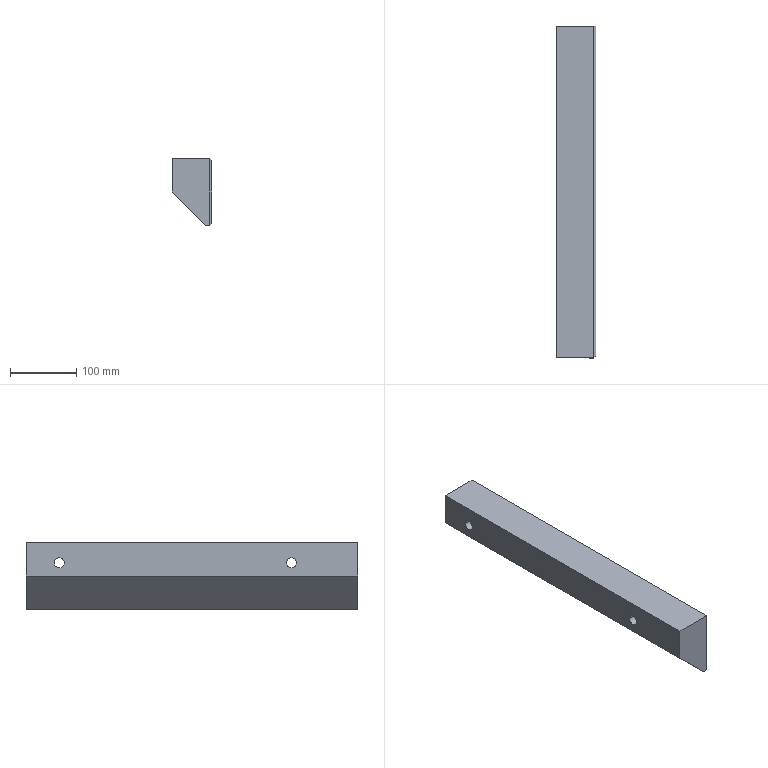Part | SolidWorks | features BaseBody 1 | 1 solid | 18 faces | box 60 x 500 x 100 mm | volume 2348382 mm3 | plane 10 | cone 4 | cylinder 4 | commonest cylinder face diameters 15 x4
STEP:
#1=CARTESIAN_POINT('',(125.077,156.249,507.107));
#2=VERTEX_POINT('',#1);
#3=CARTESIAN_POINT('',(122.077,153.249,510.107));
#4=VERTEX_POINT('',#3);
#5=CARTESIAN_POINT('',(257.41,288.582,374.773));
#6=DIRECTION('',(-0.5774,-0.5774,0.5774));
#7=VECTOR('',#6,1000.);
#8=LINE('',#5,#7);
#9=EDGE_CURVE('',#2,#4,#8,.T.);
#10=ORIENTED_EDGE('',*,*,#9,.T.);
#11=CARTESIAN_POINT('',(122.077,153.249,410.107));
#12=VERTEX_POINT('',#11);
#13=CARTESIAN_POINT('',(122.077,153.249,510.107));
#14=DIRECTION('',(0.,0.,1.));
#15=VECTOR('',#14,1000.);
#16=LINE('',#13,#15);
#17=EDGE_CURVE('',#12,#4,#16,.T.);
#18=ORIENTED_EDGE('',*,*,#17,.F.);
#19=CARTESIAN_POINT('',(125.077,156.249,413.107));
#20=VERTEX_POINT('',#19);
#21=CARTESIAN_POINT('',(124.077,155.249,412.107));
#22=DIRECTION('',(-0.5774,-0.5774,-0.5774));
#23=VECTOR('',#22,1000.);
#24=LINE('',#21,#23);
#25=EDGE_CURVE('',#20,#12,#24,.T.);
#26=ORIENTED_EDGE('',*,*,#25,.F.);
#27=CARTESIAN_POINT('',(125.077,156.249,410.107));
#28=DIRECTION('',(0.,0.,-1.));
#29=VECTOR('',#28,1000.);
#30=LINE('',#27,#29);
#31=EDGE_CURVE('',#2,#20,#30,.T.);
#32=ORIENTED_EDGE('',*,*,#31,.F.);
#33=EDGE_LOOP('',(#10,#18,#26,#32));
#34=FACE_OUTER_BOUND('',#33,.T.);
#35=CARTESIAN_POINT('',(125.077,156.249,410.107));
#36=DIRECTION('',(0.7071,-0.7071,0.));
#37=DIRECTION('',(0.,0.,-1.));
#38=AXIS2_PLACEMENT_3D('',#35,#36,#37);
#39=PLANE('',#38);
#40=ADVANCED_FACE('',(#34),#39,.T.);
#41=CARTESIAN_POINT('',(122.077,260.749,480.107));
#42=VERTEX_POINT('',#41);
#43=CARTESIAN_POINT('',(122.077,245.749,480.107));
#44=VERTEX_POINT('',#43);
#45=CARTESIAN_POINT('',(122.077,253.249,480.107));
#46=DIRECTION('',(1.,0.,0.));
#47=DIRECTION('',(0.,1.,0.));
#48=AXIS2_PLACEMENT_3D('',#45,#46,#47);
#49=CIRCLE('',#48,7.5);
#50=EDGE_CURVE('',#42,#44,#49,.T.);
#51=ORIENTED_EDGE('',*,*,#50,.F.);
#52=CARTESIAN_POINT('',(125.077,263.749,480.107));
#53=VERTEX_POINT('',#52);
#54=CARTESIAN_POINT('',(122.077,260.749,480.107));
#55=DIRECTION('',(0.7071,0.7071,0.));
#56=VECTOR('',#55,1000.);
#57=LINE('',#54,#56);
#58=EDGE_CURVE('',#42,#53,#57,.T.);
#59=ORIENTED_EDGE('',*,*,#58,.T.);
#60=CARTESIAN_POINT('',(125.077,242.749,480.107));
#61=VERTEX_POINT('',#60);
#62=CARTESIAN_POINT('',(125.077,253.249,480.107));
#63=DIRECTION('',(-1.,0.,0.));
#64=DIRECTION('',(0.,1.,0.));
#65=AXIS2_PLACEMENT_3D('',#62,#63,#64);
#66=CIRCLE('',#65,10.5);
#67=EDGE_CURVE('',#61,#53,#66,.T.);
#68=ORIENTED_EDGE('',*,*,#67,.F.);
#69=CARTESIAN_POINT('',(122.077,245.749,480.107));
#70=DIRECTION('',(0.7071,-0.7071,0.));
#71=VECTOR('',#70,1000.);
#72=LINE('',#69,#71);
#73=EDGE_CURVE('',#44,#61,#72,.T.);
#74=ORIENTED_EDGE('',*,*,#73,.F.);
#75=EDGE_LOOP('',(#51,#59,#68,#74));
#76=FACE_OUTER_BOUND('',#75,.T.);
#77=CARTESIAN_POINT('',(122.077,253.249,480.107));
#78=DIRECTION('',(1.,0.,0.));
#79=DIRECTION('',(0.,1.,0.));
#80=AXIS2_PLACEMENT_3D('',#77,#78,#79);
#81=CONICAL_SURFACE('',#80,7.5,0.7854);
#82=ADVANCED_FACE('',(#76),#81,.F.);
#83=ORIENTED_EDGE('',*,*,#58,.F.);
#84=CARTESIAN_POINT('',(122.077,253.249,480.107));
#85=DIRECTION('',(1.,0.,0.));
#86=DIRECTION('',(0.,1.,0.));
#87=AXIS2_PLACEMENT_3D('',#84,#85,#86);
#88=CIRCLE('',#87,7.5);
#89=EDGE_CURVE('',#44,#42,#88,.T.);
#90=ORIENTED_EDGE('',*,*,#89,.F.);
#91=ORIENTED_EDGE('',*,*,#73,.T.);
#92=CARTESIAN_POINT('',(125.077,253.249,480.107));
#93=DIRECTION('',(-1.,0.,0.));
#94=DIRECTION('',(0.,1.,0.));
#95=AXIS2_PLACEMENT_3D('',#92,#93,#94);
#96=CIRCLE('',#95,10.5);
#97=EDGE_CURVE('',#53,#61,#96,.T.);
#98=ORIENTED_EDGE('',*,*,#97,.F.);
#99=EDGE_LOOP('',(#83,#90,#91,#98));
#100=FACE_OUTER_BOUND('',#99,.T.);
#101=CARTESIAN_POINT('',(122.077,253.249,480.107));
#102=DIRECTION('',(1.,0.,0.));
#103=DIRECTION('',(0.,1.,0.));
#104=AXIS2_PLACEMENT_3D('',#101,#102,#103);
#105=CONICAL_SURFACE('',#104,7.5,0.7854);
#106=ADVANCED_FACE('',(#100),#105,.F.);
#107=CARTESIAN_POINT('',(65.077,260.749,480.107));
#108=VERTEX_POINT('',#107);
#109=CARTESIAN_POINT('',(65.077,260.749,480.107));
#110=DIRECTION('',(1.,0.,0.));
#111=VECTOR('',#110,1000.);
#112=LINE('',#109,#111);
#113=EDGE_CURVE('',#108,#42,#112,.T.);
#114=ORIENTED_EDGE('',*,*,#113,.F.);
#115=CARTESIAN_POINT('',(65.077,245.749,480.107));
#116=VERTEX_POINT('',#115);
#117=CARTESIAN_POINT('',(65.077,253.249,480.107));
#118=DIRECTION('',(1.,0.,0.));
#119=DIRECTION('',(0.,-1.,0.));
#120=AXIS2_PLACEMENT_3D('',#117,#118,#119);
#121=CIRCLE('',#120,7.5);
#122=EDGE_CURVE('',#116,#108,#121,.T.);
#123=ORIENTED_EDGE('',*,*,#122,.F.);
#124=CARTESIAN_POINT('',(65.077,245.749,480.107));
#125=DIRECTION('',(1.,0.,0.));
#126=VECTOR('',#125,1000.);
#127=LINE('',#124,#126);
#128=EDGE_CURVE('',#116,#44,#127,.T.);
#129=ORIENTED_EDGE('',*,*,#128,.T.);
#130=ORIENTED_EDGE('',*,*,#89,.T.);
#131=EDGE_LOOP('',(#114,#123,#129,#130));
#132=FACE_OUTER_BOUND('',#131,.T.);
#133=CARTESIAN_POINT('',(65.077,253.249,480.107));
#134=DIRECTION('',(1.,0.,0.));
#135=DIRECTION('',(0.,1.,0.));
#136=AXIS2_PLACEMENT_3D('',#133,#134,#135);
#137=CYLINDRICAL_SURFACE('',#136,7.5);
#138=ADVANCED_FACE('',(#132),#137,.F.);
#139=CARTESIAN_POINT('',(65.077,253.249,480.107));
#140=DIRECTION('',(1.,0.,0.));
#141=DIRECTION('',(0.,-1.,0.));
#142=AXIS2_PLACEMENT_3D('',#139,#140,#141);
#143=CIRCLE('',#142,7.5);
#144=EDGE_CURVE('',#108,#116,#143,.T.);
#145=ORIENTED_EDGE('',*,*,#144,.F.);
#146=ORIENTED_EDGE('',*,*,#113,.T.);
#147=ORIENTED_EDGE('',*,*,#50,.T.);
#148=ORIENTED_EDGE('',*,*,#128,.F.);
#149=EDGE_LOOP('',(#145,#146,#147,#148));
#150=FACE_OUTER_BOUND('',#149,.T.);
#151=CARTESIAN_POINT('',(65.077,253.249,480.107));
#152=DIRECTION('',(1.,0.,0.));
#153=DIRECTION('',(0.,1.,0.));
#154=AXIS2_PLACEMENT_3D('',#151,#152,#153);
#155=CYLINDRICAL_SURFACE('',#154,7.5);
#156=ADVANCED_FACE('',(#150),#155,.F.);
#157=CARTESIAN_POINT('',(115.077,153.249,410.107));
#158=VERTEX_POINT('',#157);
#159=CARTESIAN_POINT('',(115.077,153.249,410.107));
#160=DIRECTION('',(-1.,0.,0.));
#161=VECTOR('',#160,1000.);
#162=LINE('',#159,#161);
#163=EDGE_CURVE('',#12,#158,#162,.T.);
#164=ORIENTED_EDGE('',*,*,#163,.F.);
#165=ORIENTED_EDGE('',*,*,#17,.T.);
#166=CARTESIAN_POINT('',(65.077,153.249,510.107));
#167=VERTEX_POINT('',#166);
#168=CARTESIAN_POINT('',(125.077,153.249,510.107));
#169=DIRECTION('',(1.,0.,0.));
#170=VECTOR('',#169,1000.);
#171=LINE('',#168,#170);
#172=EDGE_CURVE('',#167,#4,#171,.T.);
#173=ORIENTED_EDGE('',*,*,#172,.F.);
#174=CARTESIAN_POINT('',(65.077,153.249,460.107));
#175=VERTEX_POINT('',#174);
#176=CARTESIAN_POINT('',(65.077,153.249,510.107));
#177=DIRECTION('',(0.,0.,1.));
#178=VECTOR('',#177,1000.);
#179=LINE('',#176,#178);
#180=EDGE_CURVE('',#175,#167,#179,.T.);
#181=ORIENTED_EDGE('',*,*,#180,.F.);
#182=CARTESIAN_POINT('',(65.077,153.249,460.107));
#183=DIRECTION('',(-0.7071,0.,0.7071));
#184=VECTOR('',#183,1000.);
#185=LINE('',#182,#184);
#186=EDGE_CURVE('',#158,#175,#185,.T.);
#187=ORIENTED_EDGE('',*,*,#186,.F.);
#188=EDGE_LOOP('',(#164,#165,#173,#181,#187));
#189=FACE_OUTER_BOUND('',#188,.T.);
#190=CARTESIAN_POINT('',(125.077,153.249,410.107));
#191=DIRECTION('',(0.,-1.,0.));
#192=DIRECTION('',(0.,0.,-1.));
#193=AXIS2_PLACEMENT_3D('',#190,#191,#192);
#194=PLANE('',#193);
#195=ADVANCED_FACE('',(#189),#194,.T.);
#196=CARTESIAN_POINT('',(122.077,653.249,510.107));
#197=VERTEX_POINT('',#196);
#198=CARTESIAN_POINT('',(122.077,803.249,510.107));
#199=DIRECTION('',(0.,1.,0.));
#200=VECTOR('',#199,1000.);
#201=LINE('',#198,#200);
#202=EDGE_CURVE('',#4,#197,#201,.T.);
#203=ORIENTED_EDGE('',*,*,#202,.F.);
#204=ORIENTED_EDGE('',*,*,#9,.F.);
#205=CARTESIAN_POINT('',(125.077,653.249,507.107));
#206=VERTEX_POINT('',#205);
#207=CARTESIAN_POINT('',(125.077,803.249,507.107));
#208=DIRECTION('',(0.,-1.,0.));
#209=VECTOR('',#208,1000.);
#210=LINE('',#207,#209);
#211=EDGE_CURVE('',#206,#2,#210,.T.);
#212=ORIENTED_EDGE('',*,*,#211,.F.);
#213=CARTESIAN_POINT('',(125.077,653.249,507.107));
#214=DIRECTION('',(-0.7071,0.,0.7071));
#215=VECTOR('',#214,1000.);
#216=LINE('',#213,#215);
#217=EDGE_CURVE('',#206,#197,#216,.T.);
#218=ORIENTED_EDGE('',*,*,#217,.T.);
#219=EDGE_LOOP('',(#203,#204,#212,#218));
#220=FACE_OUTER_BOUND('',#219,.T.);
#221=CARTESIAN_POINT('',(125.077,803.249,507.107));
#222=DIRECTION('',(-0.7071,0.,-0.7071));
#223=DIRECTION('',(-0.7071,0.,0.7071));
#224=AXIS2_PLACEMENT_3D('',#221,#222,#223);
#225=PLANE('',#224);
#226=ADVANCED_FACE('',(#220),#225,.F.);
#227=CARTESIAN_POINT('',(125.077,653.249,413.107));
#228=VERTEX_POINT('',#227);
#229=CARTESIAN_POINT('',(125.077,803.249,413.107));
#230=DIRECTION('',(0.,1.,0.));
#231=VECTOR('',#230,1000.);
#232=LINE('',#229,#231);
#233=EDGE_CURVE('',#20,#228,#232,.T.);
#234=ORIENTED_EDGE('',*,*,#233,.F.);
#235=ORIENTED_EDGE('',*,*,#25,.T.);
#236=CARTESIAN_POINT('',(122.077,653.249,410.107));
#237=VERTEX_POINT('',#236);
#238=CARTESIAN_POINT('',(122.077,803.249,410.107));
#239=DIRECTION('',(0.,-1.,0.));
#240=VECTOR('',#239,1000.);
#241=LINE('',#238,#240);
#242=EDGE_CURVE('',#237,#12,#241,.T.);
#243=ORIENTED_EDGE('',*,*,#242,.F.);
#244=CARTESIAN_POINT('',(122.077,653.249,410.107));
#245=DIRECTION('',(0.7071,0.,0.7071));
#246=VECTOR('',#245,1000.);
#247=LINE('',#244,#246);
#248=EDGE_CURVE('',#237,#228,#247,.T.);
#249=ORIENTED_EDGE('',*,*,#248,.T.);
#250=EDGE_LOOP('',(#234,#235,#243,#249));
#251=FACE_OUTER_BOUND('',#250,.T.);
#252=CARTESIAN_POINT('',(122.077,803.249,410.107));
#253=DIRECTION('',(-0.7071,0.,0.7071));
#254=DIRECTION('',(0.,1.,0.));
#255=AXIS2_PLACEMENT_3D('',#252,#253,#254);
#256=PLANE('',#255);
#257=ADVANCED_FACE('',(#251),#256,.F.);
#258=ORIENTED_EDGE('',*,*,#67,.T.);
#259=ORIENTED_EDGE('',*,*,#97,.T.);
#260=EDGE_LOOP('',(#258,#259));
#261=FACE_BOUND('',#260,.T.);
#262=CARTESIAN_POINT('',(125.077,592.749,480.107));
#263=VERTEX_POINT('',#262);
#264=CARTESIAN_POINT('',(125.077,613.749,480.107));
#265=VERTEX_POINT('',#264);
#266=CARTESIAN_POINT('',(125.077,603.249,480.107));
#267=DIRECTION('',(-1.,0.,0.));
#268=DIRECTION('',(0.,1.,0.));
#269=AXIS2_PLACEMENT_3D('',#266,#267,#268);
#270=CIRCLE('',#269,10.5);
#271=EDGE_CURVE('',#263,#265,#270,.T.);
#272=ORIENTED_EDGE('',*,*,#271,.T.);
#273=CARTESIAN_POINT('',(125.077,603.249,480.107));
#274=DIRECTION('',(-1.,0.,0.));
#275=DIRECTION('',(0.,1.,0.));
#276=AXIS2_PLACEMENT_3D('',#273,#274,#275);
#277=CIRCLE('',#276,10.5);
#278=EDGE_CURVE('',#265,#263,#277,.T.);
#279=ORIENTED_EDGE('',*,*,#278,.T.);
#280=EDGE_LOOP('',(#272,#279));
#281=FACE_BOUND('',#280,.T.);
#282=ORIENTED_EDGE('',*,*,#211,.T.);
#283=ORIENTED_EDGE('',*,*,#31,.T.);
#284=ORIENTED_EDGE('',*,*,#233,.T.);
#285=CARTESIAN_POINT('',(125.077,653.249,410.107));
#286=DIRECTION('',(0.,0.,-1.));
#287=VECTOR('',#286,1000.);
#288=LINE('',#285,#287);
#289=EDGE_CURVE('',#206,#228,#288,.T.);
#290=ORIENTED_EDGE('',*,*,#289,.F.);
#291=EDGE_LOOP('',(#282,#283,#284,#290));
#292=FACE_OUTER_BOUND('',#291,.T.);
#293=CARTESIAN_POINT('',(125.077,803.249,410.107));
#294=DIRECTION('',(-1.,0.,0.));
#295=DIRECTION('',(0.,0.,1.));
#296=AXIS2_PLACEMENT_3D('',#293,#294,#295);
#297=PLANE('',#296);
#298=ADVANCED_FACE('',(#261,#281,#292),#297,.F.);
#299=ORIENTED_EDGE('',*,*,#122,.T.);
#300=ORIENTED_EDGE('',*,*,#144,.T.);
#301=EDGE_LOOP('',(#299,#300));
#302=FACE_BOUND('',#301,.T.);
#303=CARTESIAN_POINT('',(65.077,595.749,480.107));
#304=VERTEX_POINT('',#303);
#305=CARTESIAN_POINT('',(65.077,610.749,480.107));
#306=VERTEX_POINT('',#305);
#307=CARTESIAN_POINT('',(65.077,603.249,480.107));
#308=DIRECTION('',(1.,0.,0.));
#309=DIRECTION('',(0.,-1.,0.));
#310=AXIS2_PLACEMENT_3D('',#307,#308,#309);
#311=CIRCLE('',#310,7.5);
#312=EDGE_CURVE('',#304,#306,#311,.T.);
#313=ORIENTED_EDGE('',*,*,#312,.T.);
#314=CARTESIAN_POINT('',(65.077,603.249,480.107));
#315=DIRECTION('',(1.,0.,0.));
#316=DIRECTION('',(0.,-1.,0.));
#317=AXIS2_PLACEMENT_3D('',#314,#315,#316);
#318=CIRCLE('',#317,7.5);
#319=EDGE_CURVE('',#306,#304,#318,.T.);
#320=ORIENTED_EDGE('',*,*,#319,.T.);
#321=EDGE_LOOP('',(#313,#320));
#322=FACE_BOUND('',#321,.T.);
#323=CARTESIAN_POINT('',(65.077,653.249,460.107));
#324=VERTEX_POINT('',#323);
#325=CARTESIAN_POINT('',(65.077,803.249,460.107));
#326=DIRECTION('',(0.,-1.,0.));
#327=VECTOR('',#326,1000.);
#328=LINE('',#325,#327);
#329=EDGE_CURVE('',#324,#175,#328,.T.);
#330=ORIENTED_EDGE('',*,*,#329,.T.);
#331=ORIENTED_EDGE('',*,*,#180,.T.);
#332=CARTESIAN_POINT('',(65.077,653.249,510.107));
#333=VERTEX_POINT('',#332);
#334=CARTESIAN_POINT('',(65.077,803.249,510.107));
#335=DIRECTION('',(0.,-1.,0.));
#336=VECTOR('',#335,1000.);
#337=LINE('',#334,#336);
#338=EDGE_CURVE('',#333,#167,#337,.T.);
#339=ORIENTED_EDGE('',*,*,#338,.F.);
#340=CARTESIAN_POINT('',(65.077,653.249,510.107));
#341=DIRECTION('',(0.,0.,-1.));
#342=VECTOR('',#341,1000.);
#343=LINE('',#340,#342);
#344=EDGE_CURVE('',#333,#324,#343,.T.);
#345=ORIENTED_EDGE('',*,*,#344,.T.);
#346=EDGE_LOOP('',(#330,#331,#339,#345));
#347=FACE_OUTER_BOUND('',#346,.T.);
#348=CARTESIAN_POINT('',(65.077,803.249,510.107));
#349=DIRECTION('',(1.,0.,0.));
#350=DIRECTION('',(0.,1.,0.));
#351=AXIS2_PLACEMENT_3D('',#348,#349,#350);
#352=PLANE('',#351);
#353=ADVANCED_FACE('',(#302,#322,#347),#352,.F.);
#354=CARTESIAN_POINT('',(115.077,653.249,410.107));
#355=VERTEX_POINT('',#354);
#356=CARTESIAN_POINT('',(115.077,803.249,410.107));
#357=DIRECTION('',(0.,-1.,0.));
#358=VECTOR('',#357,1000.);
#359=LINE('',#356,#358);
#360=EDGE_CURVE('',#355,#158,#359,.T.);
#361=ORIENTED_EDGE('',*,*,#360,.T.);
#362=ORIENTED_EDGE('',*,*,#186,.T.);
#363=ORIENTED_EDGE('',*,*,#329,.F.);
#364=CARTESIAN_POINT('',(65.077,653.249,460.107));
#365=DIRECTION('',(-0.7071,0.,0.7071));
#366=VECTOR('',#365,1000.);
#367=LINE('',#364,#366);
#368=EDGE_CURVE('',#355,#324,#367,.T.);
#369=ORIENTED_EDGE('',*,*,#368,.F.);
#370=EDGE_LOOP('',(#361,#362,#363,#369));
#371=FACE_OUTER_BOUND('',#370,.T.);
#372=CARTESIAN_POINT('',(65.077,803.249,460.107));
#373=DIRECTION('',(0.7071,0.,0.7071));
#374=DIRECTION('',(0.,-1.,0.));
#375=AXIS2_PLACEMENT_3D('',#372,#373,#374);
#376=PLANE('',#375);
#377=ADVANCED_FACE('',(#371),#376,.F.);
#378=ORIENTED_EDGE('',*,*,#242,.T.);
#379=ORIENTED_EDGE('',*,*,#163,.T.);
#380=ORIENTED_EDGE('',*,*,#360,.F.);
#381=CARTESIAN_POINT('',(115.077,653.249,410.107));
#382=DIRECTION('',(1.,0.,0.));
#383=VECTOR('',#382,1000.);
#384=LINE('',#381,#383);
#385=EDGE_CURVE('',#355,#237,#384,.T.);
#386=ORIENTED_EDGE('',*,*,#385,.T.);
#387=EDGE_LOOP('',(#378,#379,#380,#386));
#388=FACE_OUTER_BOUND('',#387,.T.);
#389=CARTESIAN_POINT('',(115.077,803.249,410.107));
#390=DIRECTION('',(0.,0.,1.));
#391=DIRECTION('',(1.,0.,0.));
#392=AXIS2_PLACEMENT_3D('',#389,#390,#391);
#393=PLANE('',#392);
#394=ADVANCED_FACE('',(#388),#393,.F.);
#395=ORIENTED_EDGE('',*,*,#338,.T.);
#396=ORIENTED_EDGE('',*,*,#172,.T.);
#397=ORIENTED_EDGE('',*,*,#202,.T.);
#398=CARTESIAN_POINT('',(-977.923,653.249,510.107));
#399=DIRECTION('',(-1.,0.,0.));
#400=VECTOR('',#399,1000.);
#401=LINE('',#398,#400);
#402=EDGE_CURVE('',#197,#333,#401,.T.);
#403=ORIENTED_EDGE('',*,*,#402,.T.);
#404=EDGE_LOOP('',(#395,#396,#397,#403));
#405=FACE_OUTER_BOUND('',#404,.T.);
#406=CARTESIAN_POINT('',(125.077,803.249,510.107));
#407=DIRECTION('',(0.,0.,-1.));
#408=DIRECTION('',(0.,-1.,0.));
#409=AXIS2_PLACEMENT_3D('',#406,#407,#408);
#410=PLANE('',#409);
#411=ADVANCED_FACE('',(#405),#410,.F.);
#412=ORIENTED_EDGE('',*,*,#402,.F.);
#413=ORIENTED_EDGE('',*,*,#217,.F.);
#414=ORIENTED_EDGE('',*,*,#289,.T.);
#415=ORIENTED_EDGE('',*,*,#248,.F.);
#416=ORIENTED_EDGE('',*,*,#385,.F.);
#417=ORIENTED_EDGE('',*,*,#368,.T.);
#418=ORIENTED_EDGE('',*,*,#344,.F.);
#419=EDGE_LOOP('',(#412,#413,#414,#415,#416,#417,#418));
#420=FACE_OUTER_BOUND('',#419,.T.);
#421=CARTESIAN_POINT('',(-977.923,653.249,510.107));
#422=DIRECTION('',(0.,-1.,0.));
#423=DIRECTION('',(0.,0.,-1.));
#424=AXIS2_PLACEMENT_3D('',#421,#422,#423);
#425=PLANE('',#424);
#426=ADVANCED_FACE('',(#420),#425,.F.);
#427=CARTESIAN_POINT('',(122.077,610.749,480.107));
#428=VERTEX_POINT('',#427);
#429=CARTESIAN_POINT('',(65.077,610.749,480.107));
#430=DIRECTION('',(1.,0.,0.));
#431=VECTOR('',#430,1000.);
#432=LINE('',#429,#431);
#433=EDGE_CURVE('',#306,#428,#432,.T.);
#434=ORIENTED_EDGE('',*,*,#433,.F.);
#435=ORIENTED_EDGE('',*,*,#312,.F.);
#436=CARTESIAN_POINT('',(122.077,595.749,480.107));
#437=VERTEX_POINT('',#436);
#438=CARTESIAN_POINT('',(65.077,595.749,480.107));
#439=DIRECTION('',(1.,0.,0.));
#440=VECTOR('',#439,1000.);
#441=LINE('',#438,#440);
#442=EDGE_CURVE('',#304,#437,#441,.T.);
#443=ORIENTED_EDGE('',*,*,#442,.T.);
#444=CARTESIAN_POINT('',(122.077,603.249,480.107));
#445=DIRECTION('',(1.,0.,0.));
#446=DIRECTION('',(0.,1.,0.));
#447=AXIS2_PLACEMENT_3D('',#444,#445,#446);
#448=CIRCLE('',#447,7.5);
#449=EDGE_CURVE('',#437,#428,#448,.T.);
#450=ORIENTED_EDGE('',*,*,#449,.T.);
#451=EDGE_LOOP('',(#434,#435,#443,#450));
#452=FACE_OUTER_BOUND('',#451,.T.);
#453=CARTESIAN_POINT('',(65.077,603.249,480.107));
#454=DIRECTION('',(1.,0.,0.));
#455=DIRECTION('',(0.,1.,0.));
#456=AXIS2_PLACEMENT_3D('',#453,#454,#455);
#457=CYLINDRICAL_SURFACE('',#456,7.5);
#458=ADVANCED_FACE('',(#452),#457,.F.);
#459=ORIENTED_EDGE('',*,*,#319,.F.);
#460=ORIENTED_EDGE('',*,*,#433,.T.);
#461=CARTESIAN_POINT('',(122.077,603.249,480.107));
#462=DIRECTION('',(1.,0.,0.));
#463=DIRECTION('',(0.,1.,0.));
#464=AXIS2_PLACEMENT_3D('',#461,#462,#463);
#465=CIRCLE('',#464,7.5);
#466=EDGE_CURVE('',#428,#437,#465,.T.);
#467=ORIENTED_EDGE('',*,*,#466,.T.);
#468=ORIENTED_EDGE('',*,*,#442,.F.);
#469=EDGE_LOOP('',(#459,#460,#467,#468));
#470=FACE_OUTER_BOUND('',#469,.T.);
#471=CARTESIAN_POINT('',(65.077,603.249,480.107));
#472=DIRECTION('',(1.,0.,0.));
#473=DIRECTION('',(0.,1.,0.));
#474=AXIS2_PLACEMENT_3D('',#471,#472,#473);
#475=CYLINDRICAL_SURFACE('',#474,7.5);
#476=ADVANCED_FACE('',(#470),#475,.F.);
#477=ORIENTED_EDGE('',*,*,#466,.F.);
#478=CARTESIAN_POINT('',(122.077,610.749,480.107));
#479=DIRECTION('',(0.7071,0.7071,0.));
#480=VECTOR('',#479,1000.);
#481=LINE('',#478,#480);
#482=EDGE_CURVE('',#428,#265,#481,.T.);
#483=ORIENTED_EDGE('',*,*,#482,.T.);
#484=ORIENTED_EDGE('',*,*,#271,.F.);
#485=CARTESIAN_POINT('',(122.077,595.749,480.107));
#486=DIRECTION('',(0.7071,-0.7071,0.));
#487=VECTOR('',#486,1000.);
#488=LINE('',#485,#487);
#489=EDGE_CURVE('',#437,#263,#488,.T.);
#490=ORIENTED_EDGE('',*,*,#489,.F.);
#491=EDGE_LOOP('',(#477,#483,#484,#490));
#492=FACE_OUTER_BOUND('',#491,.T.);
#493=CARTESIAN_POINT('',(122.077,603.249,480.107));
#494=DIRECTION('',(1.,0.,0.));
#495=DIRECTION('',(0.,1.,0.));
#496=AXIS2_PLACEMENT_3D('',#493,#494,#495);
#497=CONICAL_SURFACE('',#496,7.5,0.7854);
#498=ADVANCED_FACE('',(#492),#497,.F.);
#499=ORIENTED_EDGE('',*,*,#482,.F.);
#500=ORIENTED_EDGE('',*,*,#449,.F.);
#501=ORIENTED_EDGE('',*,*,#489,.T.);
#502=ORIENTED_EDGE('',*,*,#278,.F.);
#503=EDGE_LOOP('',(#499,#500,#501,#502));
#504=FACE_OUTER_BOUND('',#503,.T.);
#505=CARTESIAN_POINT('',(122.077,603.249,480.107));
#506=DIRECTION('',(1.,0.,0.));
#507=DIRECTION('',(0.,1.,0.));
#508=AXIS2_PLACEMENT_3D('',#505,#506,#507);
#509=CONICAL_SURFACE('',#508,7.5,0.7854);
#510=ADVANCED_FACE('',(#504),#509,.F.);
#511=CLOSED_SHELL('',(#40,#82,#106,#138,#156,#195,#226,#257,#298,#353,#377,#394,#411,#426,#458,#476,#498,#510));
#512=MANIFOLD_SOLID_BREP('',#511);
#513=CARTESIAN_POINT('',(0.,0.,0.));
#514=DIRECTION('',(0.,0.,1.));
#515=DIRECTION('',(1.,0.,0.));
#516=AXIS2_PLACEMENT_3D('',#513,#514,#515);
#517=(LENGTH_UNIT()NAMED_UNIT(*)SI_UNIT(.MILLI.,.METRE.));
#518=UNCERTAINTY_MEASURE_WITH_UNIT(LENGTH_MEASURE(0.00001),#517,'','');
#519=(NAMED_UNIT(*)PLANE_ANGLE_UNIT()SI_UNIT($,.RADIAN.));
#520=(NAMED_UNIT(*)SI_UNIT($,.STERADIAN.)SOLID_ANGLE_UNIT());
#521=(GEOMETRIC_REPRESENTATION_CONTEXT(3)GLOBAL_UNCERTAINTY_ASSIGNED_CONTEXT((#518))GLOBAL_UNIT_ASSIGNED_CONTEXT((#517,#519,#520))REPRESENTATION_CONTEXT('',''));
#522=ADVANCED_BREP_SHAPE_REPRESENTATION('',(#512,#516),#521);